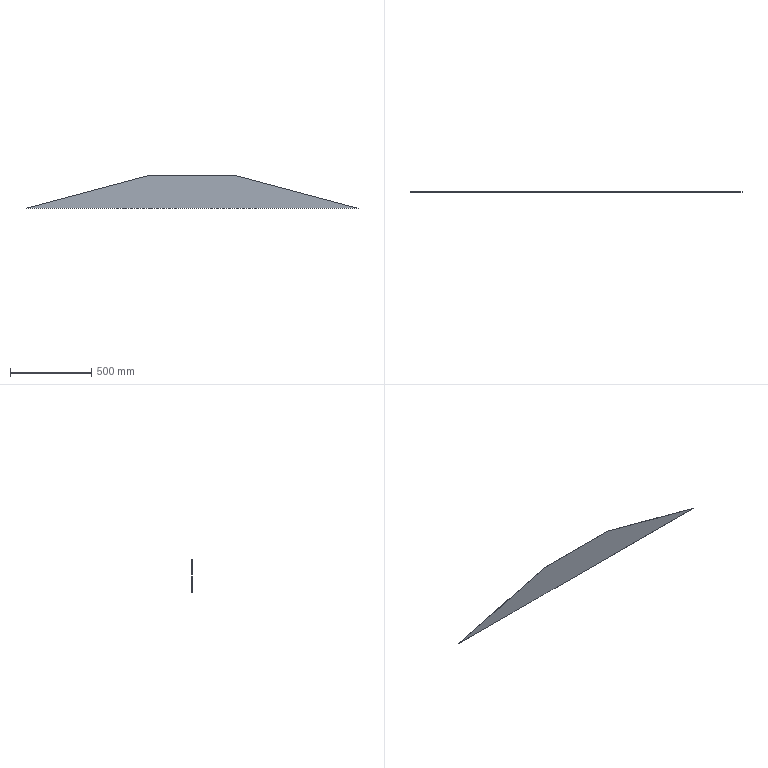Part | SolidWorks | features FlatPattern 1, SMBaseFlange 1, SheetMetal 1 | 1 solid | 6 faces | box 2043 x 1.2 x 200 mm | volume 311138 mm3 | plane 6
STEP:
#1=CARTESIAN_POINT('',(275.,0.,0.));
#2=VERTEX_POINT('',#1);
#3=CARTESIAN_POINT('',(1021.41,0.,-200.));
#4=VERTEX_POINT('',#3);
#5=CARTESIAN_POINT('',(275.,0.,0.));
#6=DIRECTION('',(0.9659,0.,-0.2588));
#7=VECTOR('',#6,1000.);
#8=LINE('',#5,#7);
#9=EDGE_CURVE('',#2,#4,#8,.T.);
#10=ORIENTED_EDGE('',*,*,#9,.F.);
#11=CARTESIAN_POINT('',(275.,-1.2,0.));
#12=VERTEX_POINT('',#11);
#13=CARTESIAN_POINT('',(275.,-1.2,0.));
#14=DIRECTION('',(0.,1.,0.));
#15=VECTOR('',#14,1000.);
#16=LINE('',#13,#15);
#17=EDGE_CURVE('',#12,#2,#16,.T.);
#18=ORIENTED_EDGE('',*,*,#17,.F.);
#19=CARTESIAN_POINT('',(1021.41,-1.2,-200.));
#20=VERTEX_POINT('',#19);
#21=CARTESIAN_POINT('',(275.,-1.2,0.));
#22=DIRECTION('',(0.9659,0.,-0.2588));
#23=VECTOR('',#22,1000.);
#24=LINE('',#21,#23);
#25=EDGE_CURVE('',#12,#20,#24,.T.);
#26=ORIENTED_EDGE('',*,*,#25,.T.);
#27=CARTESIAN_POINT('',(1021.41,-1.2,-200.));
#28=DIRECTION('',(0.,1.,0.));
#29=VECTOR('',#28,1000.);
#30=LINE('',#27,#29);
#31=EDGE_CURVE('',#20,#4,#30,.T.);
#32=ORIENTED_EDGE('',*,*,#31,.T.);
#33=EDGE_LOOP('',(#10,#18,#26,#32));
#34=FACE_OUTER_BOUND('',#33,.T.);
#35=CARTESIAN_POINT('',(275.,-1.2,0.));
#36=DIRECTION('',(0.2588,0.,0.9659));
#37=DIRECTION('',(0.9659,0.,-0.2588));
#38=AXIS2_PLACEMENT_3D('',#35,#36,#37);
#39=PLANE('',#38);
#40=ADVANCED_FACE('',(#34),#39,.T.);
#41=CARTESIAN_POINT('',(-275.,0.,0.));
#42=VERTEX_POINT('',#41);
#43=CARTESIAN_POINT('',(-275.,0.,0.));
#44=DIRECTION('',(1.,0.,0.));
#45=VECTOR('',#44,1000.);
#46=LINE('',#43,#45);
#47=EDGE_CURVE('',#42,#2,#46,.T.);
#48=ORIENTED_EDGE('',*,*,#47,.F.);
#49=CARTESIAN_POINT('',(-275.,-1.2,0.));
#50=VERTEX_POINT('',#49);
#51=CARTESIAN_POINT('',(-275.,-1.2,0.));
#52=DIRECTION('',(0.,1.,0.));
#53=VECTOR('',#52,1000.);
#54=LINE('',#51,#53);
#55=EDGE_CURVE('',#50,#42,#54,.T.);
#56=ORIENTED_EDGE('',*,*,#55,.F.);
#57=CARTESIAN_POINT('',(-275.,-1.2,0.));
#58=DIRECTION('',(1.,0.,0.));
#59=VECTOR('',#58,1000.);
#60=LINE('',#57,#59);
#61=EDGE_CURVE('',#50,#12,#60,.T.);
#62=ORIENTED_EDGE('',*,*,#61,.T.);
#63=ORIENTED_EDGE('',*,*,#17,.T.);
#64=EDGE_LOOP('',(#48,#56,#62,#63));
#65=FACE_OUTER_BOUND('',#64,.T.);
#66=CARTESIAN_POINT('',(-275.,-1.2,0.));
#67=DIRECTION('',(0.,0.,1.));
#68=DIRECTION('',(1.,0.,0.));
#69=AXIS2_PLACEMENT_3D('',#66,#67,#68);
#70=PLANE('',#69);
#71=ADVANCED_FACE('',(#65),#70,.T.);
#72=CARTESIAN_POINT('',(-1021.41,0.,-200.));
#73=VERTEX_POINT('',#72);
#74=CARTESIAN_POINT('',(-275.,0.,0.));
#75=DIRECTION('',(0.9659,0.,0.2588));
#76=VECTOR('',#75,1000.);
#77=LINE('',#74,#76);
#78=EDGE_CURVE('',#73,#42,#77,.T.);
#79=ORIENTED_EDGE('',*,*,#78,.F.);
#80=CARTESIAN_POINT('',(-1021.41,-1.2,-200.));
#81=VERTEX_POINT('',#80);
#82=CARTESIAN_POINT('',(-1021.41,-1.2,-200.));
#83=DIRECTION('',(0.,1.,0.));
#84=VECTOR('',#83,1000.);
#85=LINE('',#82,#84);
#86=EDGE_CURVE('',#81,#73,#85,.T.);
#87=ORIENTED_EDGE('',*,*,#86,.F.);
#88=CARTESIAN_POINT('',(-275.,-1.2,0.));
#89=DIRECTION('',(0.9659,0.,0.2588));
#90=VECTOR('',#89,1000.);
#91=LINE('',#88,#90);
#92=EDGE_CURVE('',#81,#50,#91,.T.);
#93=ORIENTED_EDGE('',*,*,#92,.T.);
#94=ORIENTED_EDGE('',*,*,#55,.T.);
#95=EDGE_LOOP('',(#79,#87,#93,#94));
#96=FACE_OUTER_BOUND('',#95,.T.);
#97=CARTESIAN_POINT('',(-275.,-1.2,0.));
#98=DIRECTION('',(-0.2588,0.,0.9659));
#99=DIRECTION('',(0.9659,0.,0.2588));
#100=AXIS2_PLACEMENT_3D('',#97,#98,#99);
#101=PLANE('',#100);
#102=ADVANCED_FACE('',(#96),#101,.T.);
#103=CARTESIAN_POINT('',(-1021.41,0.,-200.));
#104=DIRECTION('',(-1.,0.,0.));
#105=VECTOR('',#104,1000.);
#106=LINE('',#103,#105);
#107=EDGE_CURVE('',#4,#73,#106,.T.);
#108=ORIENTED_EDGE('',*,*,#107,.F.);
#109=ORIENTED_EDGE('',*,*,#31,.F.);
#110=CARTESIAN_POINT('',(-1021.41,-1.2,-200.));
#111=DIRECTION('',(-1.,0.,0.));
#112=VECTOR('',#111,1000.);
#113=LINE('',#110,#112);
#114=EDGE_CURVE('',#20,#81,#113,.T.);
#115=ORIENTED_EDGE('',*,*,#114,.T.);
#116=ORIENTED_EDGE('',*,*,#86,.T.);
#117=EDGE_LOOP('',(#108,#109,#115,#116));
#118=FACE_OUTER_BOUND('',#117,.T.);
#119=CARTESIAN_POINT('',(-1021.41,-1.2,-200.));
#120=DIRECTION('',(0.,0.,-1.));
#121=DIRECTION('',(-1.,0.,0.));
#122=AXIS2_PLACEMENT_3D('',#119,#120,#121);
#123=PLANE('',#122);
#124=ADVANCED_FACE('',(#118),#123,.T.);
#125=ORIENTED_EDGE('',*,*,#25,.F.);
#126=ORIENTED_EDGE('',*,*,#61,.F.);
#127=ORIENTED_EDGE('',*,*,#92,.F.);
#128=ORIENTED_EDGE('',*,*,#114,.F.);
#129=EDGE_LOOP('',(#125,#126,#127,#128));
#130=FACE_OUTER_BOUND('',#129,.T.);
#131=CARTESIAN_POINT('',(0.,-1.2,0.));
#132=DIRECTION('',(0.,1.,0.));
#133=DIRECTION('',(0.,0.,1.));
#134=AXIS2_PLACEMENT_3D('',#131,#132,#133);
#135=PLANE('',#134);
#136=ADVANCED_FACE('',(#130),#135,.F.);
#137=ORIENTED_EDGE('',*,*,#9,.T.);
#138=ORIENTED_EDGE('',*,*,#107,.T.);
#139=ORIENTED_EDGE('',*,*,#78,.T.);
#140=ORIENTED_EDGE('',*,*,#47,.T.);
#141=EDGE_LOOP('',(#137,#138,#139,#140));
#142=FACE_OUTER_BOUND('',#141,.T.);
#143=CARTESIAN_POINT('',(0.,0.,0.));
#144=DIRECTION('',(0.,1.,0.));
#145=DIRECTION('',(0.,0.,1.));
#146=AXIS2_PLACEMENT_3D('',#143,#144,#145);
#147=PLANE('',#146);
#148=ADVANCED_FACE('',(#142),#147,.T.);
#149=CLOSED_SHELL('',(#40,#71,#102,#124,#136,#148));
#150=MANIFOLD_SOLID_BREP('',#149);
#151=CARTESIAN_POINT('',(0.,0.,0.));
#152=DIRECTION('',(0.,0.,1.));
#153=DIRECTION('',(1.,0.,0.));
#154=AXIS2_PLACEMENT_3D('',#151,#152,#153);
#155=(LENGTH_UNIT()NAMED_UNIT(*)SI_UNIT(.MILLI.,.METRE.));
#156=UNCERTAINTY_MEASURE_WITH_UNIT(LENGTH_MEASURE(0.00001),#155,'','');
#157=(NAMED_UNIT(*)PLANE_ANGLE_UNIT()SI_UNIT($,.RADIAN.));
#158=(NAMED_UNIT(*)SI_UNIT($,.STERADIAN.)SOLID_ANGLE_UNIT());
#159=(GEOMETRIC_REPRESENTATION_CONTEXT(3)GLOBAL_UNCERTAINTY_ASSIGNED_CONTEXT((#156))GLOBAL_UNIT_ASSIGNED_CONTEXT((#155,#157,#158))REPRESENTATION_CONTEXT('',''));
#160=ADVANCED_BREP_SHAPE_REPRESENTATION('',(#150,#154),#159);